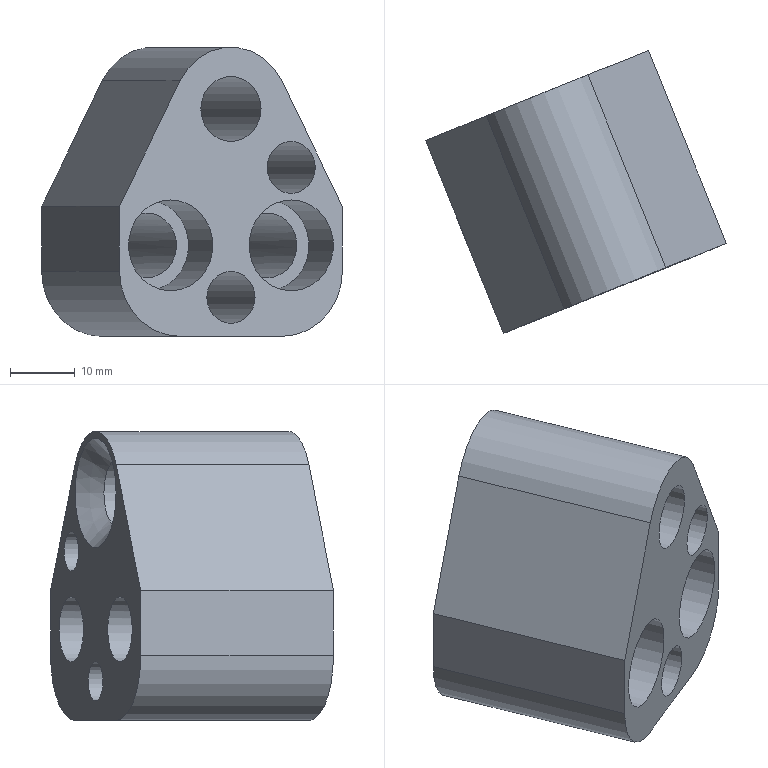Part | NX | features solid 2 | 1 solid | 24 faces | box 46.293 x 43.53 x 44.5 mm | volume 29019 mm3 | cylinder 12 | plane 11 | cone 1 | commonest cylinder face diameters 10 x3 6 x2 8 x2 14 x2 20 x2 19 x1
STEP:
#1=CARTESIAN_POINT('',(-687.987,326.31,69.209));
#2=VERTEX_POINT('',#1);
#3=CARTESIAN_POINT('',(-691.696,324.811,69.209));
#4=DIRECTION('',(-0.3746,0.9272,0.));
#5=DIRECTION('',(0.9272,0.3746,0.));
#6=AXIS2_PLACEMENT_3D('',#3,#4,#5);
#7=CIRCLE('',#6,4.);
#8=EDGE_CURVE('',#2,#2,#7,.F.);
#9=ORIENTED_EDGE('',*,*,#8,.F.);
#10=EDGE_LOOP('',(#9));
#11=FACE_BOUND('',#10,.T.);
#12=CARTESIAN_POINT('',(-700.968,321.065,70.209));
#13=VERTEX_POINT('',#12);
#14=CARTESIAN_POINT('',(-700.968,321.065,77.209));
#15=DIRECTION('',(0.3746,-0.9272,0.));
#16=DIRECTION('',(0.,0.,-1.));
#17=AXIS2_PLACEMENT_3D('',#14,#15,#16);
#18=CIRCLE('',#17,7.);
#19=EDGE_CURVE('',#13,#13,#18,.T.);
#20=ORIENTED_EDGE('',*,*,#19,.F.);
#21=EDGE_LOOP('',(#20));
#22=FACE_BOUND('',#21,.T.);
#23=CARTESIAN_POINT('',(-682.424,328.557,70.209));
#24=VERTEX_POINT('',#23);
#25=CARTESIAN_POINT('',(-682.424,328.557,77.209));
#26=DIRECTION('',(0.3746,-0.9272,0.));
#27=DIRECTION('',(0.,0.,-1.));
#28=AXIS2_PLACEMENT_3D('',#25,#26,#27);
#29=CIRCLE('',#28,7.);
#30=EDGE_CURVE('',#24,#24,#29,.T.);
#31=ORIENTED_EDGE('',*,*,#30,.F.);
#32=EDGE_LOOP('',(#31));
#33=FACE_BOUND('',#32,.T.);
#34=CARTESIAN_POINT('',(-687.06,326.684,98.209));
#35=VERTEX_POINT('',#34);
#36=CARTESIAN_POINT('',(-691.696,324.811,98.209));
#37=DIRECTION('',(-0.3746,0.9272,0.));
#38=DIRECTION('',(0.9272,0.3746,0.));
#39=AXIS2_PLACEMENT_3D('',#36,#37,#38);
#40=CIRCLE('',#39,5.);
#41=EDGE_CURVE('',#35,#35,#40,.T.);
#42=ORIENTED_EDGE('',*,*,#41,.T.);
#43=EDGE_LOOP('',(#42));
#44=FACE_BOUND('',#43,.T.);
#45=CARTESIAN_POINT('',(-708.849,317.881,73.209));
#46=VERTEX_POINT('',#45);
#47=CARTESIAN_POINT('',(-699.577,321.627,63.209));
#48=VERTEX_POINT('',#47);
#49=CARTESIAN_POINT('',(-699.577,321.627,73.209));
#50=DIRECTION('',(0.3746,-0.9272,0.));
#51=DIRECTION('',(0.,0.,-1.));
#52=AXIS2_PLACEMENT_3D('',#49,#50,#51);
#53=CIRCLE('',#52,10.);
#54=EDGE_CURVE('',#46,#48,#53,.T.);
#55=ORIENTED_EDGE('',*,*,#54,.T.);
#56=CARTESIAN_POINT('',(-683.815,327.995,63.209));
#57=VERTEX_POINT('',#56);
#58=CARTESIAN_POINT('',(-683.815,327.995,63.209));
#59=DIRECTION('',(-0.9272,-0.3746,0.));
#60=VECTOR('',#59,1000.);
#61=LINE('',#58,#60);
#62=EDGE_CURVE('',#57,#48,#61,.T.);
#63=ORIENTED_EDGE('',*,*,#62,.F.);
#64=CARTESIAN_POINT('',(-674.543,331.741,73.209));
#65=VERTEX_POINT('',#64);
#66=CARTESIAN_POINT('',(-683.815,327.995,73.209));
#67=DIRECTION('',(0.3746,-0.9272,0.));
#68=DIRECTION('',(0.,0.,-1.));
#69=AXIS2_PLACEMENT_3D('',#66,#67,#68);
#70=CIRCLE('',#69,10.);
#71=EDGE_CURVE('',#57,#65,#70,.T.);
#72=ORIENTED_EDGE('',*,*,#71,.T.);
#73=CARTESIAN_POINT('',(-674.543,331.741,83.209));
#74=VERTEX_POINT('',#73);
#75=CARTESIAN_POINT('',(-674.543,331.741,83.209));
#76=DIRECTION('',(0.,0.,-1.));
#77=VECTOR('',#76,1000.);
#78=LINE('',#75,#77);
#79=EDGE_CURVE('',#74,#65,#78,.T.);
#80=ORIENTED_EDGE('',*,*,#79,.F.);
#81=CARTESIAN_POINT('',(-683.88,327.969,102.59));
#82=VERTEX_POINT('',#81);
#83=CARTESIAN_POINT('',(-683.88,327.969,102.59));
#84=DIRECTION('',(0.4275,0.1727,-0.8874));
#85=VECTOR('',#84,1000.);
#86=LINE('',#83,#85);
#87=EDGE_CURVE('',#82,#74,#86,.T.);
#88=ORIENTED_EDGE('',*,*,#87,.F.);
#89=CARTESIAN_POINT('',(-699.512,321.653,102.59));
#90=VERTEX_POINT('',#89);
#91=CARTESIAN_POINT('',(-691.696,324.811,98.209));
#92=DIRECTION('',(0.3746,-0.9272,0.));
#93=DIRECTION('',(0.,0.,-1.));
#94=AXIS2_PLACEMENT_3D('',#91,#92,#93);
#95=CIRCLE('',#94,9.5);
#96=EDGE_CURVE('',#82,#90,#95,.T.);
#97=ORIENTED_EDGE('',*,*,#96,.T.);
#98=CARTESIAN_POINT('',(-708.849,317.881,83.209));
#99=VERTEX_POINT('',#98);
#100=CARTESIAN_POINT('',(-699.512,321.653,102.59));
#101=DIRECTION('',(-0.4275,-0.1727,-0.8874));
#102=VECTOR('',#101,1000.);
#103=LINE('',#100,#102);
#104=EDGE_CURVE('',#90,#99,#103,.T.);
#105=ORIENTED_EDGE('',*,*,#104,.T.);
#106=CARTESIAN_POINT('',(-708.849,317.881,83.209));
#107=DIRECTION('',(0.,0.,-1.));
#108=VECTOR('',#107,1000.);
#109=LINE('',#106,#108);
#110=EDGE_CURVE('',#99,#46,#109,.T.);
#111=ORIENTED_EDGE('',*,*,#110,.T.);
#112=EDGE_LOOP('',(#55,#63,#72,#80,#88,#97,#105,#111));
#113=FACE_BOUND('',#112,.T.);
#114=CARTESIAN_POINT('',(-678.715,330.056,89.209));
#115=VERTEX_POINT('',#114);
#116=CARTESIAN_POINT('',(-682.424,328.557,89.209));
#117=DIRECTION('',(-0.3746,0.9272,0.));
#118=DIRECTION('',(0.9272,0.3746,0.));
#119=AXIS2_PLACEMENT_3D('',#116,#117,#118);
#120=CIRCLE('',#119,4.);
#121=EDGE_CURVE('',#115,#115,#120,.F.);
#122=ORIENTED_EDGE('',*,*,#121,.F.);
#123=EDGE_LOOP('',(#122));
#124=FACE_BOUND('',#123,.T.);
#125=CARTESIAN_POINT('',(-699.577,321.627,73.209));
#126=DIRECTION('',(0.3746,-0.9272,0.));
#127=DIRECTION('',(-0.9272,-0.3746,0.));
#128=AXIS2_PLACEMENT_3D('',#125,#126,#127);
#129=PLANE('',#128);
#130=ADVANCED_FACE('',(#11,#22,#33,#44,#113,#124),#129,.T.);
#131=CARTESIAN_POINT('',(-712.955,350.735,72.209));
#132=VERTEX_POINT('',#131);
#133=CARTESIAN_POINT('',(-712.955,350.735,77.209));
#134=DIRECTION('',(0.3746,-0.9272,0.));
#135=DIRECTION('',(0.,0.,-1.));
#136=AXIS2_PLACEMENT_3D('',#133,#134,#135);
#137=CIRCLE('',#136,5.);
#138=EDGE_CURVE('',#132,#132,#137,.T.);
#139=ORIENTED_EDGE('',*,*,#138,.F.);
#140=EDGE_LOOP('',(#139));
#141=FACE_BOUND('',#140,.T.);
#142=CARTESIAN_POINT('',(-709.35,328.464,77.209));
#143=VERTEX_POINT('',#142);
#144=CARTESIAN_POINT('',(-704.714,330.337,77.209));
#145=DIRECTION('',(0.3746,-0.9272,0.));
#146=DIRECTION('',(-0.9272,-0.3746,0.));
#147=AXIS2_PLACEMENT_3D('',#144,#145,#146);
#148=CIRCLE('',#147,5.);
#149=EDGE_CURVE('',#143,#143,#148,.T.);
#150=ORIENTED_EDGE('',*,*,#149,.T.);
#151=EDGE_LOOP('',(#150));
#152=FACE_BOUND('',#151,.T.);
#153=CARTESIAN_POINT('',(-700.968,321.065,77.209));
#154=DIRECTION('',(-0.3746,0.9272,0.));
#155=DIRECTION('',(0.9272,0.3746,0.));
#156=AXIS2_PLACEMENT_3D('',#153,#154,#155);
#157=CYLINDRICAL_SURFACE('',#156,5.);
#158=ADVANCED_FACE('',(#141,#152),#157,.F.);
#159=CARTESIAN_POINT('',(-694.411,358.227,72.209));
#160=VERTEX_POINT('',#159);
#161=CARTESIAN_POINT('',(-694.411,358.227,77.209));
#162=DIRECTION('',(0.3746,-0.9272,0.));
#163=DIRECTION('',(0.,0.,-1.));
#164=AXIS2_PLACEMENT_3D('',#161,#162,#163);
#165=CIRCLE('',#164,5.);
#166=EDGE_CURVE('',#160,#160,#165,.T.);
#167=ORIENTED_EDGE('',*,*,#166,.F.);
#168=EDGE_LOOP('',(#167));
#169=FACE_BOUND('',#168,.T.);
#170=CARTESIAN_POINT('',(-690.806,335.956,77.209));
#171=VERTEX_POINT('',#170);
#172=CARTESIAN_POINT('',(-686.17,337.829,77.209));
#173=DIRECTION('',(0.3746,-0.9272,0.));
#174=DIRECTION('',(-0.9272,-0.3746,0.));
#175=AXIS2_PLACEMENT_3D('',#172,#173,#174);
#176=CIRCLE('',#175,5.);
#177=EDGE_CURVE('',#171,#171,#176,.T.);
#178=ORIENTED_EDGE('',*,*,#177,.T.);
#179=EDGE_LOOP('',(#178));
#180=FACE_BOUND('',#179,.T.);
#181=CARTESIAN_POINT('',(-682.424,328.557,77.209));
#182=DIRECTION('',(-0.3746,0.9272,0.));
#183=DIRECTION('',(0.9272,0.3746,0.));
#184=AXIS2_PLACEMENT_3D('',#181,#182,#183);
#185=CYLINDRICAL_SURFACE('',#184,5.);
#186=ADVANCED_FACE('',(#169,#180),#185,.F.);
#187=CARTESIAN_POINT('',(-694.411,358.227,86.209));
#188=VERTEX_POINT('',#187);
#189=CARTESIAN_POINT('',(-694.411,358.227,89.209));
#190=DIRECTION('',(0.3746,-0.9272,0.));
#191=DIRECTION('',(0.,0.,-1.));
#192=AXIS2_PLACEMENT_3D('',#189,#190,#191);
#193=CIRCLE('',#192,3.);
#194=EDGE_CURVE('',#188,#188,#193,.T.);
#195=ORIENTED_EDGE('',*,*,#194,.T.);
#196=EDGE_LOOP('',(#195));
#197=FACE_BOUND('',#196,.T.);
#198=ORIENTED_EDGE('',*,*,#166,.T.);
#199=EDGE_LOOP('',(#198));
#200=FACE_BOUND('',#199,.T.);
#201=CARTESIAN_POINT('',(-711.471,351.334,98.209));
#202=VERTEX_POINT('',#201);
#203=CARTESIAN_POINT('',(-703.683,354.481,98.209));
#204=DIRECTION('',(0.3746,-0.9272,0.));
#205=DIRECTION('',(-0.9272,-0.3746,0.));
#206=AXIS2_PLACEMENT_3D('',#203,#204,#205);
#207=CIRCLE('',#206,8.4);
#208=EDGE_CURVE('',#202,#202,#207,.T.);
#209=ORIENTED_EDGE('',*,*,#208,.T.);
#210=EDGE_LOOP('',(#209));
#211=FACE_BOUND('',#210,.T.);
#212=CARTESIAN_POINT('',(-720.836,347.551,73.209));
#213=VERTEX_POINT('',#212);
#214=CARTESIAN_POINT('',(-711.564,351.297,63.209));
#215=VERTEX_POINT('',#214);
#216=CARTESIAN_POINT('',(-711.564,351.297,73.209));
#217=DIRECTION('',(0.3746,-0.9272,0.));
#218=DIRECTION('',(0.,0.,-1.));
#219=AXIS2_PLACEMENT_3D('',#216,#217,#218);
#220=CIRCLE('',#219,10.);
#221=EDGE_CURVE('',#213,#215,#220,.T.);
#222=ORIENTED_EDGE('',*,*,#221,.F.);
#223=CARTESIAN_POINT('',(-720.836,347.551,83.209));
#224=VERTEX_POINT('',#223);
#225=CARTESIAN_POINT('',(-720.836,347.551,83.209));
#226=DIRECTION('',(0.,0.,-1.));
#227=VECTOR('',#226,1000.);
#228=LINE('',#225,#227);
#229=EDGE_CURVE('',#224,#213,#228,.T.);
#230=ORIENTED_EDGE('',*,*,#229,.F.);
#231=CARTESIAN_POINT('',(-711.499,351.323,102.59));
#232=VERTEX_POINT('',#231);
#233=CARTESIAN_POINT('',(-711.499,351.323,102.59));
#234=DIRECTION('',(-0.4275,-0.1727,-0.8874));
#235=VECTOR('',#234,1000.);
#236=LINE('',#233,#235);
#237=EDGE_CURVE('',#232,#224,#236,.T.);
#238=ORIENTED_EDGE('',*,*,#237,.F.);
#239=CARTESIAN_POINT('',(-695.867,357.639,102.59));
#240=VERTEX_POINT('',#239);
#241=CARTESIAN_POINT('',(-703.683,354.481,98.209));
#242=DIRECTION('',(0.3746,-0.9272,0.));
#243=DIRECTION('',(0.,0.,-1.));
#244=AXIS2_PLACEMENT_3D('',#241,#242,#243);
#245=CIRCLE('',#244,9.5);
#246=EDGE_CURVE('',#240,#232,#245,.T.);
#247=ORIENTED_EDGE('',*,*,#246,.F.);
#248=CARTESIAN_POINT('',(-686.53,361.411,83.209));
#249=VERTEX_POINT('',#248);
#250=CARTESIAN_POINT('',(-695.867,357.639,102.59));
#251=DIRECTION('',(0.4275,0.1727,-0.8874));
#252=VECTOR('',#251,1000.);
#253=LINE('',#250,#252);
#254=EDGE_CURVE('',#240,#249,#253,.T.);
#255=ORIENTED_EDGE('',*,*,#254,.T.);
#256=CARTESIAN_POINT('',(-686.53,361.411,73.209));
#257=VERTEX_POINT('',#256);
#258=CARTESIAN_POINT('',(-686.53,361.411,83.209));
#259=DIRECTION('',(0.,0.,-1.));
#260=VECTOR('',#259,1000.);
#261=LINE('',#258,#260);
#262=EDGE_CURVE('',#249,#257,#261,.T.);
#263=ORIENTED_EDGE('',*,*,#262,.T.);
#264=CARTESIAN_POINT('',(-695.802,357.665,63.209));
#265=VERTEX_POINT('',#264);
#266=CARTESIAN_POINT('',(-695.802,357.665,73.209));
#267=DIRECTION('',(0.3746,-0.9272,0.));
#268=DIRECTION('',(0.,0.,-1.));
#269=AXIS2_PLACEMENT_3D('',#266,#267,#268);
#270=CIRCLE('',#269,10.);
#271=EDGE_CURVE('',#265,#257,#270,.T.);
#272=ORIENTED_EDGE('',*,*,#271,.F.);
#273=CARTESIAN_POINT('',(-695.802,357.665,63.209));
#274=DIRECTION('',(-0.9272,-0.3746,0.));
#275=VECTOR('',#274,1000.);
#276=LINE('',#273,#275);
#277=EDGE_CURVE('',#265,#215,#276,.T.);
#278=ORIENTED_EDGE('',*,*,#277,.T.);
#279=EDGE_LOOP('',(#222,#230,#238,#247,#255,#263,#272,#278));
#280=FACE_BOUND('',#279,.T.);
#281=ORIENTED_EDGE('',*,*,#138,.T.);
#282=EDGE_LOOP('',(#281));
#283=FACE_BOUND('',#282,.T.);
#284=CARTESIAN_POINT('',(-703.683,354.481,66.209));
#285=VERTEX_POINT('',#284);
#286=CARTESIAN_POINT('',(-703.683,354.481,69.209));
#287=DIRECTION('',(0.3746,-0.9272,0.));
#288=DIRECTION('',(0.,0.,-1.));
#289=AXIS2_PLACEMENT_3D('',#286,#287,#288);
#290=CIRCLE('',#289,3.);
#291=EDGE_CURVE('',#285,#285,#290,.T.);
#292=ORIENTED_EDGE('',*,*,#291,.T.);
#293=EDGE_LOOP('',(#292));
#294=FACE_BOUND('',#293,.T.);
#295=CARTESIAN_POINT('',(-711.564,351.297,73.209));
#296=DIRECTION('',(0.3746,-0.9272,0.));
#297=DIRECTION('',(-0.9272,-0.3746,0.));
#298=AXIS2_PLACEMENT_3D('',#295,#296,#297);
#299=PLANE('',#298);
#300=ADVANCED_FACE('',(#197,#200,#211,#280,#283,#294),#299,.F.);
#301=ORIENTED_EDGE('',*,*,#221,.T.);
#302=CARTESIAN_POINT('',(-699.577,321.627,63.209));
#303=DIRECTION('',(-0.3746,0.9272,0.));
#304=VECTOR('',#303,1000.);
#305=LINE('',#302,#304);
#306=EDGE_CURVE('',#48,#215,#305,.T.);
#307=ORIENTED_EDGE('',*,*,#306,.F.);
#308=ORIENTED_EDGE('',*,*,#54,.F.);
#309=CARTESIAN_POINT('',(-708.849,317.881,73.209));
#310=DIRECTION('',(-0.3746,0.9272,0.));
#311=VECTOR('',#310,1000.);
#312=LINE('',#309,#311);
#313=EDGE_CURVE('',#46,#213,#312,.T.);
#314=ORIENTED_EDGE('',*,*,#313,.T.);
#315=EDGE_LOOP('',(#301,#307,#308,#314));
#316=FACE_BOUND('',#315,.T.);
#317=CARTESIAN_POINT('',(-699.577,321.627,73.209));
#318=DIRECTION('',(-0.3746,0.9272,0.));
#319=DIRECTION('',(0.9272,0.3746,0.));
#320=AXIS2_PLACEMENT_3D('',#317,#318,#319);
#321=CYLINDRICAL_SURFACE('',#320,10.);
#322=ADVANCED_FACE('',(#316),#321,.T.);
#323=ORIENTED_EDGE('',*,*,#277,.F.);
#324=CARTESIAN_POINT('',(-683.815,327.995,63.209));
#325=DIRECTION('',(-0.3746,0.9272,0.));
#326=VECTOR('',#325,1000.);
#327=LINE('',#324,#326);
#328=EDGE_CURVE('',#57,#265,#327,.T.);
#329=ORIENTED_EDGE('',*,*,#328,.F.);
#330=ORIENTED_EDGE('',*,*,#62,.T.);
#331=ORIENTED_EDGE('',*,*,#306,.T.);
#332=EDGE_LOOP('',(#323,#329,#330,#331));
#333=FACE_BOUND('',#332,.T.);
#334=CARTESIAN_POINT('',(-683.815,327.995,63.209));
#335=DIRECTION('',(0.,0.,-1.));
#336=DIRECTION('',(-0.9272,-0.3746,0.));
#337=AXIS2_PLACEMENT_3D('',#334,#335,#336);
#338=PLANE('',#337);
#339=ADVANCED_FACE('',(#333),#338,.T.);
#340=ORIENTED_EDGE('',*,*,#271,.T.);
#341=CARTESIAN_POINT('',(-674.543,331.741,73.209));
#342=DIRECTION('',(-0.3746,0.9272,0.));
#343=VECTOR('',#342,1000.);
#344=LINE('',#341,#343);
#345=EDGE_CURVE('',#65,#257,#344,.T.);
#346=ORIENTED_EDGE('',*,*,#345,.F.);
#347=ORIENTED_EDGE('',*,*,#71,.F.);
#348=ORIENTED_EDGE('',*,*,#328,.T.);
#349=EDGE_LOOP('',(#340,#346,#347,#348));
#350=FACE_BOUND('',#349,.T.);
#351=CARTESIAN_POINT('',(-683.815,327.995,73.209));
#352=DIRECTION('',(-0.3746,0.9272,0.));
#353=DIRECTION('',(0.9272,0.3746,0.));
#354=AXIS2_PLACEMENT_3D('',#351,#352,#353);
#355=CYLINDRICAL_SURFACE('',#354,10.);
#356=ADVANCED_FACE('',(#350),#355,.T.);
#357=ORIENTED_EDGE('',*,*,#262,.F.);
#358=CARTESIAN_POINT('',(-674.543,331.741,83.209));
#359=DIRECTION('',(-0.3746,0.9272,0.));
#360=VECTOR('',#359,1000.);
#361=LINE('',#358,#360);
#362=EDGE_CURVE('',#74,#249,#361,.T.);
#363=ORIENTED_EDGE('',*,*,#362,.F.);
#364=ORIENTED_EDGE('',*,*,#79,.T.);
#365=ORIENTED_EDGE('',*,*,#345,.T.);
#366=EDGE_LOOP('',(#357,#363,#364,#365));
#367=FACE_BOUND('',#366,.T.);
#368=CARTESIAN_POINT('',(-674.543,331.741,83.209));
#369=DIRECTION('',(0.9272,0.3746,0.));
#370=DIRECTION('',(0.3746,-0.9272,0.));
#371=AXIS2_PLACEMENT_3D('',#368,#369,#370);
#372=PLANE('',#371);
#373=ADVANCED_FACE('',(#367),#372,.T.);
#374=ORIENTED_EDGE('',*,*,#254,.F.);
#375=CARTESIAN_POINT('',(-683.88,327.969,102.59));
#376=DIRECTION('',(-0.3746,0.9272,0.));
#377=VECTOR('',#376,1000.);
#378=LINE('',#375,#377);
#379=EDGE_CURVE('',#82,#240,#378,.T.);
#380=ORIENTED_EDGE('',*,*,#379,.F.);
#381=ORIENTED_EDGE('',*,*,#87,.T.);
#382=ORIENTED_EDGE('',*,*,#362,.T.);
#383=EDGE_LOOP('',(#374,#380,#381,#382));
#384=FACE_BOUND('',#383,.T.);
#385=CARTESIAN_POINT('',(-683.88,327.969,102.59));
#386=DIRECTION('',(0.8227,0.3324,0.4611));
#387=DIRECTION('',(0.4275,0.1727,-0.8874));
#388=AXIS2_PLACEMENT_3D('',#385,#386,#387);
#389=PLANE('',#388);
#390=ADVANCED_FACE('',(#384),#389,.T.);
#391=ORIENTED_EDGE('',*,*,#246,.T.);
#392=CARTESIAN_POINT('',(-699.512,321.653,102.59));
#393=DIRECTION('',(-0.3746,0.9272,0.));
#394=VECTOR('',#393,1000.);
#395=LINE('',#392,#394);
#396=EDGE_CURVE('',#90,#232,#395,.T.);
#397=ORIENTED_EDGE('',*,*,#396,.F.);
#398=ORIENTED_EDGE('',*,*,#96,.F.);
#399=ORIENTED_EDGE('',*,*,#379,.T.);
#400=EDGE_LOOP('',(#391,#397,#398,#399));
#401=FACE_BOUND('',#400,.T.);
#402=CARTESIAN_POINT('',(-691.696,324.811,98.209));
#403=DIRECTION('',(-0.3746,0.9272,0.));
#404=DIRECTION('',(0.9272,0.3746,0.));
#405=AXIS2_PLACEMENT_3D('',#402,#403,#404);
#406=CYLINDRICAL_SURFACE('',#405,9.5);
#407=ADVANCED_FACE('',(#401),#406,.T.);
#408=ORIENTED_EDGE('',*,*,#237,.T.);
#409=CARTESIAN_POINT('',(-708.849,317.881,83.209));
#410=DIRECTION('',(-0.3746,0.9272,0.));
#411=VECTOR('',#410,1000.);
#412=LINE('',#409,#411);
#413=EDGE_CURVE('',#99,#224,#412,.T.);
#414=ORIENTED_EDGE('',*,*,#413,.F.);
#415=ORIENTED_EDGE('',*,*,#104,.F.);
#416=ORIENTED_EDGE('',*,*,#396,.T.);
#417=EDGE_LOOP('',(#408,#414,#415,#416));
#418=FACE_BOUND('',#417,.T.);
#419=CARTESIAN_POINT('',(-699.512,321.653,102.59));
#420=DIRECTION('',(0.8227,0.3324,-0.4611));
#421=DIRECTION('',(-0.4275,-0.1727,-0.8874));
#422=AXIS2_PLACEMENT_3D('',#419,#420,#421);
#423=PLANE('',#422);
#424=ADVANCED_FACE('',(#418),#423,.F.);
#425=ORIENTED_EDGE('',*,*,#229,.T.);
#426=ORIENTED_EDGE('',*,*,#313,.F.);
#427=ORIENTED_EDGE('',*,*,#110,.F.);
#428=ORIENTED_EDGE('',*,*,#413,.T.);
#429=EDGE_LOOP('',(#425,#426,#427,#428));
#430=FACE_BOUND('',#429,.T.);
#431=CARTESIAN_POINT('',(-708.849,317.881,83.209));
#432=DIRECTION('',(0.9272,0.3746,0.));
#433=DIRECTION('',(0.3746,-0.9272,0.));
#434=AXIS2_PLACEMENT_3D('',#431,#432,#433);
#435=PLANE('',#434);
#436=ADVANCED_FACE('',(#430),#435,.F.);
#437=ORIENTED_EDGE('',*,*,#41,.F.);
#438=EDGE_LOOP('',(#437));
#439=FACE_BOUND('',#438,.T.);
#440=CARTESIAN_POINT('',(-697.774,353.202,98.209));
#441=VERTEX_POINT('',#440);
#442=CARTESIAN_POINT('',(-702.409,351.329,98.209));
#443=DIRECTION('',(0.3746,-0.9272,0.));
#444=DIRECTION('',(0.9272,0.3746,0.));
#445=AXIS2_PLACEMENT_3D('',#442,#443,#444);
#446=CIRCLE('',#445,5.);
#447=EDGE_CURVE('',#441,#441,#446,.T.);
#448=ORIENTED_EDGE('',*,*,#447,.F.);
#449=EDGE_LOOP('',(#448));
#450=FACE_BOUND('',#449,.T.);
#451=CARTESIAN_POINT('',(-691.696,324.811,98.209));
#452=DIRECTION('',(-0.3746,0.9272,0.));
#453=DIRECTION('',(0.9272,0.3746,0.));
#454=AXIS2_PLACEMENT_3D('',#451,#452,#453);
#455=CYLINDRICAL_SURFACE('',#454,5.);
#456=ADVANCED_FACE('',(#439,#450),#455,.F.);
#457=ORIENTED_EDGE('',*,*,#208,.F.);
#458=EDGE_LOOP('',(#457));
#459=FACE_BOUND('',#458,.T.);
#460=ORIENTED_EDGE('',*,*,#447,.T.);
#461=EDGE_LOOP('',(#460));
#462=FACE_BOUND('',#461,.T.);
#463=CARTESIAN_POINT('',(-702.409,351.329,98.209));
#464=DIRECTION('',(-0.3746,0.9272,0.));
#465=DIRECTION('',(0.9272,0.3746,0.));
#466=AXIS2_PLACEMENT_3D('',#463,#464,#465);
#467=CONICAL_SURFACE('',#466,5.,0.7854);
#468=ADVANCED_FACE('',(#459,#462),#467,.F.);
#469=CARTESIAN_POINT('',(-689.916,347.101,86.209));
#470=VERTEX_POINT('',#469);
#471=CARTESIAN_POINT('',(-689.916,347.101,89.209));
#472=DIRECTION('',(0.3746,-0.9272,0.));
#473=DIRECTION('',(0.,0.,-1.));
#474=AXIS2_PLACEMENT_3D('',#471,#472,#473);
#475=CIRCLE('',#474,3.);
#476=EDGE_CURVE('',#470,#470,#475,.T.);
#477=ORIENTED_EDGE('',*,*,#476,.T.);
#478=EDGE_LOOP('',(#477));
#479=FACE_BOUND('',#478,.T.);
#480=ORIENTED_EDGE('',*,*,#194,.F.);
#481=EDGE_LOOP('',(#480));
#482=FACE_BOUND('',#481,.T.);
#483=CARTESIAN_POINT('',(-682.424,328.557,89.209));
#484=DIRECTION('',(-0.3746,0.9272,0.));
#485=DIRECTION('',(0.9272,0.3746,0.));
#486=AXIS2_PLACEMENT_3D('',#483,#484,#485);
#487=CYLINDRICAL_SURFACE('',#486,3.);
#488=ADVANCED_FACE('',(#479,#482),#487,.F.);
#489=CARTESIAN_POINT('',(-699.188,343.355,66.209));
#490=VERTEX_POINT('',#489);
#491=CARTESIAN_POINT('',(-699.188,343.355,69.209));
#492=DIRECTION('',(0.3746,-0.9272,0.));
#493=DIRECTION('',(0.,0.,-1.));
#494=AXIS2_PLACEMENT_3D('',#491,#492,#493);
#495=CIRCLE('',#494,3.);
#496=EDGE_CURVE('',#490,#490,#495,.T.);
#497=ORIENTED_EDGE('',*,*,#496,.T.);
#498=EDGE_LOOP('',(#497));
#499=FACE_BOUND('',#498,.T.);
#500=ORIENTED_EDGE('',*,*,#291,.F.);
#501=EDGE_LOOP('',(#500));
#502=FACE_BOUND('',#501,.T.);
#503=CARTESIAN_POINT('',(-691.696,324.811,69.209));
#504=DIRECTION('',(-0.3746,0.9272,0.));
#505=DIRECTION('',(0.9272,0.3746,0.));
#506=AXIS2_PLACEMENT_3D('',#503,#504,#505);
#507=CYLINDRICAL_SURFACE('',#506,3.);
#508=ADVANCED_FACE('',(#499,#502),#507,.F.);
#509=CARTESIAN_POINT('',(-686.17,337.829,70.209));
#510=VERTEX_POINT('',#509);
#511=CARTESIAN_POINT('',(-686.17,337.829,77.209));
#512=DIRECTION('',(0.3746,-0.9272,0.));
#513=DIRECTION('',(0.,0.,-1.));
#514=AXIS2_PLACEMENT_3D('',#511,#512,#513);
#515=CIRCLE('',#514,7.);
#516=EDGE_CURVE('',#510,#510,#515,.T.);
#517=ORIENTED_EDGE('',*,*,#516,.F.);
#518=EDGE_LOOP('',(#517));
#519=FACE_BOUND('',#518,.T.);
#520=ORIENTED_EDGE('',*,*,#30,.T.);
#521=EDGE_LOOP('',(#520));
#522=FACE_BOUND('',#521,.T.);
#523=CARTESIAN_POINT('',(-686.17,337.829,77.209));
#524=DIRECTION('',(0.3746,-0.9272,0.));
#525=DIRECTION('',(-0.9272,-0.3746,0.));
#526=AXIS2_PLACEMENT_3D('',#523,#524,#525);
#527=CYLINDRICAL_SURFACE('',#526,7.);
#528=ADVANCED_FACE('',(#519,#522),#527,.F.);
#529=ORIENTED_EDGE('',*,*,#177,.F.);
#530=EDGE_LOOP('',(#529));
#531=FACE_BOUND('',#530,.T.);
#532=ORIENTED_EDGE('',*,*,#516,.T.);
#533=EDGE_LOOP('',(#532));
#534=FACE_BOUND('',#533,.T.);
#535=CARTESIAN_POINT('',(-686.17,337.829,77.209));
#536=DIRECTION('',(0.3746,-0.9272,0.));
#537=DIRECTION('',(-0.9272,-0.3746,0.));
#538=AXIS2_PLACEMENT_3D('',#535,#536,#537);
#539=PLANE('',#538);
#540=ADVANCED_FACE('',(#531,#534),#539,.T.);
#541=CARTESIAN_POINT('',(-704.714,330.337,70.209));
#542=VERTEX_POINT('',#541);
#543=CARTESIAN_POINT('',(-704.714,330.337,77.209));
#544=DIRECTION('',(0.3746,-0.9272,0.));
#545=DIRECTION('',(0.,0.,-1.));
#546=AXIS2_PLACEMENT_3D('',#543,#544,#545);
#547=CIRCLE('',#546,7.);
#548=EDGE_CURVE('',#542,#542,#547,.T.);
#549=ORIENTED_EDGE('',*,*,#548,.F.);
#550=EDGE_LOOP('',(#549));
#551=FACE_BOUND('',#550,.T.);
#552=ORIENTED_EDGE('',*,*,#19,.T.);
#553=EDGE_LOOP('',(#552));
#554=FACE_BOUND('',#553,.T.);
#555=CARTESIAN_POINT('',(-704.714,330.337,77.209));
#556=DIRECTION('',(0.3746,-0.9272,0.));
#557=DIRECTION('',(-0.9272,-0.3746,0.));
#558=AXIS2_PLACEMENT_3D('',#555,#556,#557);
#559=CYLINDRICAL_SURFACE('',#558,7.);
#560=ADVANCED_FACE('',(#551,#554),#559,.F.);
#561=ORIENTED_EDGE('',*,*,#149,.F.);
#562=EDGE_LOOP('',(#561));
#563=FACE_BOUND('',#562,.T.);
#564=ORIENTED_EDGE('',*,*,#548,.T.);
#565=EDGE_LOOP('',(#564));
#566=FACE_BOUND('',#565,.T.);
#567=CARTESIAN_POINT('',(-704.714,330.337,77.209));
#568=DIRECTION('',(0.3746,-0.9272,0.));
#569=DIRECTION('',(-0.9272,-0.3746,0.));
#570=AXIS2_PLACEMENT_3D('',#567,#568,#569);
#571=PLANE('',#570);
#572=ADVANCED_FACE('',(#563,#566),#571,.T.);
#573=CARTESIAN_POINT('',(-695.479,344.853,69.209));
#574=VERTEX_POINT('',#573);
#575=CARTESIAN_POINT('',(-699.188,343.355,69.209));
#576=DIRECTION('',(-0.3746,0.9272,0.));
#577=DIRECTION('',(0.9272,0.3746,0.));
#578=AXIS2_PLACEMENT_3D('',#575,#576,#577);
#579=CIRCLE('',#578,4.);
#580=EDGE_CURVE('',#574,#574,#579,.F.);
#581=ORIENTED_EDGE('',*,*,#580,.F.);
#582=EDGE_LOOP('',(#581));
#583=FACE_BOUND('',#582,.T.);
#584=ORIENTED_EDGE('',*,*,#8,.T.);
#585=EDGE_LOOP('',(#584));
#586=FACE_BOUND('',#585,.T.);
#587=CARTESIAN_POINT('',(-691.696,324.811,69.209));
#588=DIRECTION('',(-0.3746,0.9272,0.));
#589=DIRECTION('',(0.9272,0.3746,0.));
#590=AXIS2_PLACEMENT_3D('',#587,#588,#589);
#591=CYLINDRICAL_SURFACE('',#590,4.);
#592=ADVANCED_FACE('',(#583,#586),#591,.F.);
#593=ORIENTED_EDGE('',*,*,#580,.T.);
#594=EDGE_LOOP('',(#593));
#595=FACE_BOUND('',#594,.T.);
#596=ORIENTED_EDGE('',*,*,#496,.F.);
#597=EDGE_LOOP('',(#596));
#598=FACE_BOUND('',#597,.T.);
#599=CARTESIAN_POINT('',(-699.188,343.355,69.209));
#600=DIRECTION('',(-0.3746,0.9272,0.));
#601=DIRECTION('',(0.9272,0.3746,0.));
#602=AXIS2_PLACEMENT_3D('',#599,#600,#601);
#603=PLANE('',#602);
#604=ADVANCED_FACE('',(#595,#598),#603,.F.);
#605=CARTESIAN_POINT('',(-686.207,348.599,89.209));
#606=VERTEX_POINT('',#605);
#607=CARTESIAN_POINT('',(-689.916,347.101,89.209));
#608=DIRECTION('',(-0.3746,0.9272,0.));
#609=DIRECTION('',(0.9272,0.3746,0.));
#610=AXIS2_PLACEMENT_3D('',#607,#608,#609);
#611=CIRCLE('',#610,4.);
#612=EDGE_CURVE('',#606,#606,#611,.F.);
#613=ORIENTED_EDGE('',*,*,#612,.F.);
#614=EDGE_LOOP('',(#613));
#615=FACE_BOUND('',#614,.T.);
#616=ORIENTED_EDGE('',*,*,#121,.T.);
#617=EDGE_LOOP('',(#616));
#618=FACE_BOUND('',#617,.T.);
#619=CARTESIAN_POINT('',(-682.424,328.557,89.209));
#620=DIRECTION('',(-0.3746,0.9272,0.));
#621=DIRECTION('',(0.9272,0.3746,0.));
#622=AXIS2_PLACEMENT_3D('',#619,#620,#621);
#623=CYLINDRICAL_SURFACE('',#622,4.);
#624=ADVANCED_FACE('',(#615,#618),#623,.F.);
#625=ORIENTED_EDGE('',*,*,#612,.T.);
#626=EDGE_LOOP('',(#625));
#627=FACE_BOUND('',#626,.T.);
#628=ORIENTED_EDGE('',*,*,#476,.F.);
#629=EDGE_LOOP('',(#628));
#630=FACE_BOUND('',#629,.T.);
#631=CARTESIAN_POINT('',(-689.916,347.101,89.209));
#632=DIRECTION('',(-0.3746,0.9272,0.));
#633=DIRECTION('',(0.9272,0.3746,0.));
#634=AXIS2_PLACEMENT_3D('',#631,#632,#633);
#635=PLANE('',#634);
#636=ADVANCED_FACE('',(#627,#630),#635,.F.);
#637=CLOSED_SHELL('',(#130,#158,#186,#300,#322,#339,#356,#373,#390,#407,#424,#436,#456,#468,#488,#508,#528,#540,#560,#572,#592,#604,#624,#636));
#638=MANIFOLD_SOLID_BREP('',#637);
#639=(LENGTH_UNIT()NAMED_UNIT(*)SI_UNIT(.MILLI.,.METRE.));
#640=UNCERTAINTY_MEASURE_WITH_UNIT(LENGTH_MEASURE(0.00001),#639,'','');
#641=(NAMED_UNIT(*)PLANE_ANGLE_UNIT()SI_UNIT($,.RADIAN.));
#642=(NAMED_UNIT(*)SI_UNIT($,.STERADIAN.)SOLID_ANGLE_UNIT());
#643=(GEOMETRIC_REPRESENTATION_CONTEXT(3)GLOBAL_UNCERTAINTY_ASSIGNED_CONTEXT((#640))GLOBAL_UNIT_ASSIGNED_CONTEXT((#639,#641,#642))REPRESENTATION_CONTEXT('',''));
#644=ADVANCED_BREP_SHAPE_REPRESENTATION('',(#638),#643);